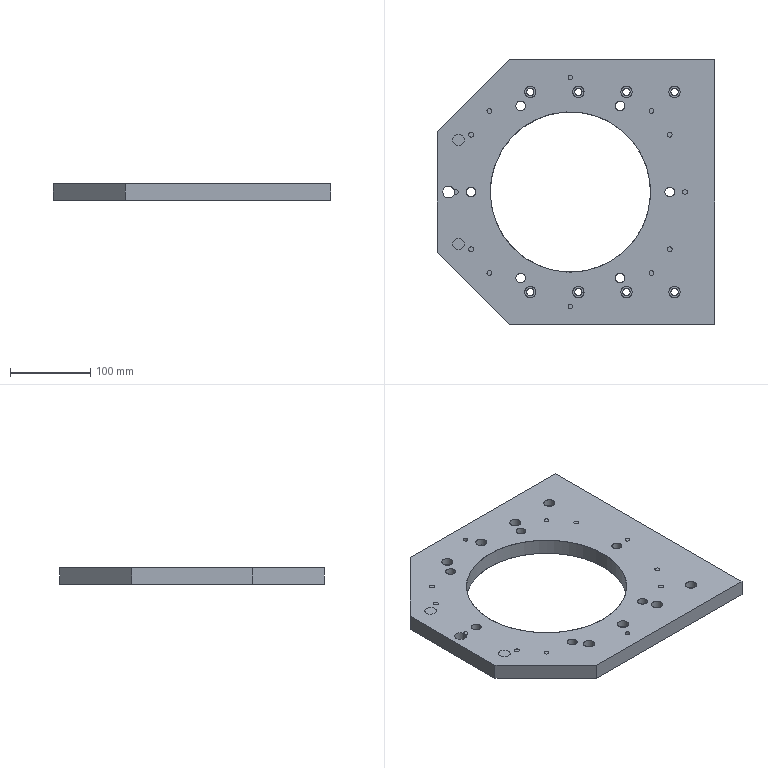NC program | NX | posted with a generic post | part box 346 x 330 x 20 mm
Lines 2745 to 2811 of 2811:
(ZLEVEL_PROFILE_COPY_COPY_1_1 , TOOL : D10JING)
N5488 T09 M6
N5490 G54
N5492 G17 G0 G90 X174.485 Y176.167 S5000 M3
N5494 G43 Z70. H9
N5496 Z-17.
N5498 G94 G1 Z-20. F1200.
N5500 X170.5 Y173.866
N5502 G3 X170. Y173. R1.
N5504 G1 Y-83.
N5506 G2 X168.536 Y-86.536 R5.
N5508 G1 X78.536 Y-176.536
N5510 G3 X78.277 Y-177.501 R1.
N5512 G1 X79.468 Y-181.946
N5514 Z-17.
N5516 G0 Z70.
N5518 X-79.468
N5520 Z-17.
N5522 G1 Z-20.
N5524 X-78.277 Y-177.501
N5526 G3 X-78.536 Y-176.536 R1.
N5528 G1 X-168.536 Y-86.536
N5530 G2 X-170. Y-83. R5.
N5532 G1 Y173.
N5534 G3 X-170.5 Y173.866 R1.
N5536 G1 X-174.485 Y176.167
N5538 Z-17.
N5540 G0 Z70.
N5542 M5
(ZLEVEL_PROFILE_COPY_COPY_COPY , TOOL : D6A45)
N5544 T07 M6
N5546 G54
N5548 G17 G0 G90 X166.904 Y175.421 S7500 M3
N5550 G43 Z70. H7
N5552 Z2.
N5554 G94 G1 Z-1. F1200.
N5556 X166.212 Y175.019
N5558 G3 X165.913 Y174.499 R0.6
N5560 G1 X165.917 Y172.986
N5562 Y-83.001
N5564 G2 X165.649 Y-83.648 R0.915
N5566 G1 X74.215 Y-175.082
N5568 X74.147 Y-175.147
N5570 G3 X73.982 Y-175.724 R0.6
N5572 G1 X74.177 Y-176.506
N5574 Z2.
N5576 G0 Z70.
N5578 X-74.177
N5580 Z2.
N5582 G1 Z-1.
N5584 X-73.982 Y-175.724
N5586 G3 X-74.147 Y-175.147 R0.6
N5588 G1 X-74.215 Y-175.082
N5590 X-165.649 Y-83.648
N5592 G2 X-165.917 Y-83.001 R0.915
N5594 G1 Y173.123
N5596 X-165.914 Y174.446
N5598 G3 X-166.213 Y174.967 R0.6
N5600 G1 X-166.925 Y175.38
N5602 Z2.
N5604 G0 Z70.
N5606 M5
N5608 M2